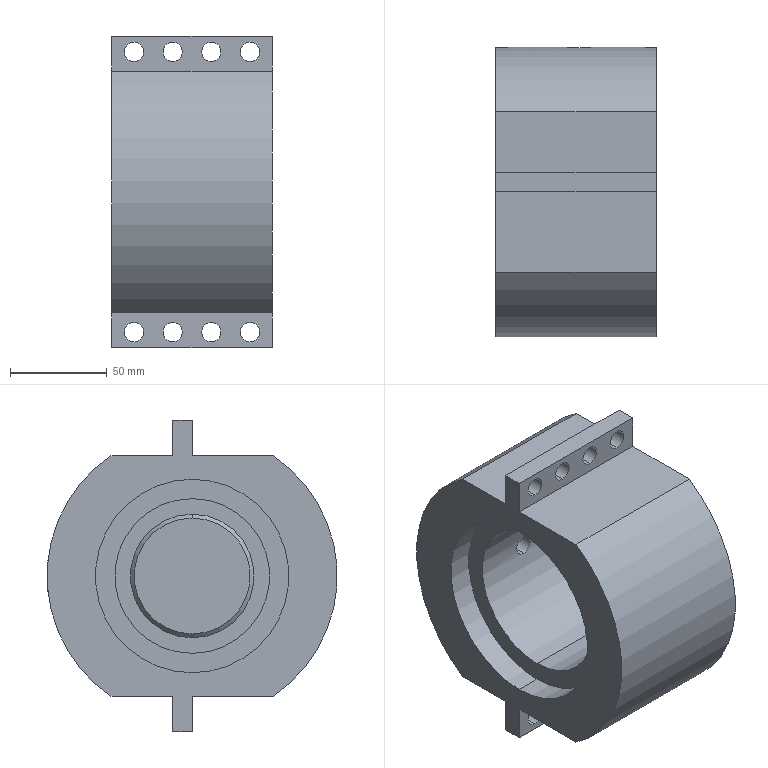Part | SolidWorks | features ICE 5, Revolution 1 | 1 solid | 44 faces | box 83 x 150 x 161 mm | volume 1012168 mm3 | cylinder 26 | plane 16 | cone 2 | commonest cylinder face diameters 10 x18 16 x2 80 x2 100 x2 150 x2